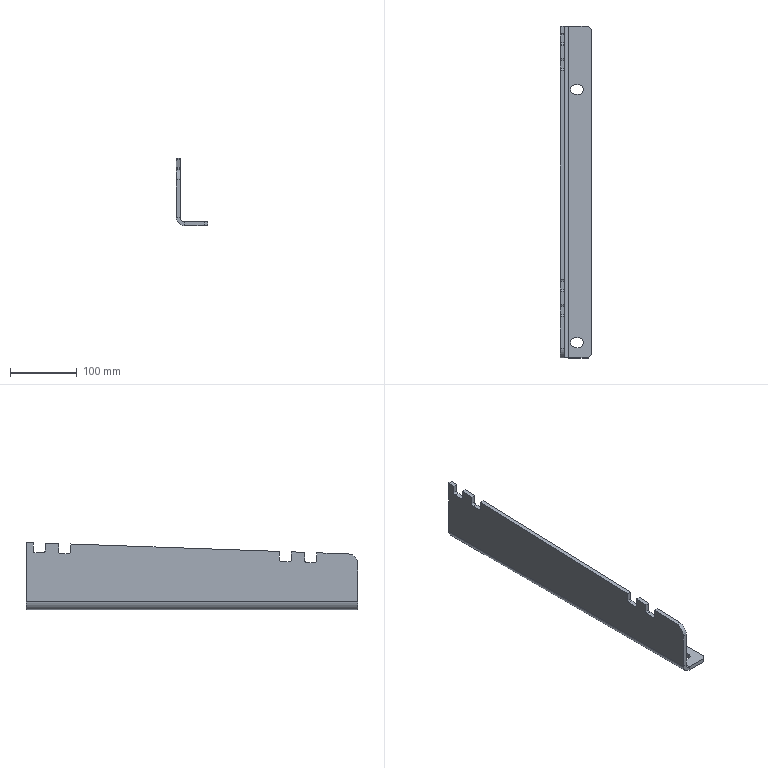Part | SolidWorks | features ICE 4, Chamfer 1, EdgeFlange 1, Fillet 1, FlatPattern 1, SMBaseFlange 1, SheetMetal 1 | 1 solid | 53 faces | box 47 x 498.4 x 101 mm | volume 376827 mm3 | plane 34 | cylinder 19 | commonest cylinder face diameters 6 x10 15 x6 12 x1 24 x1 30 x1